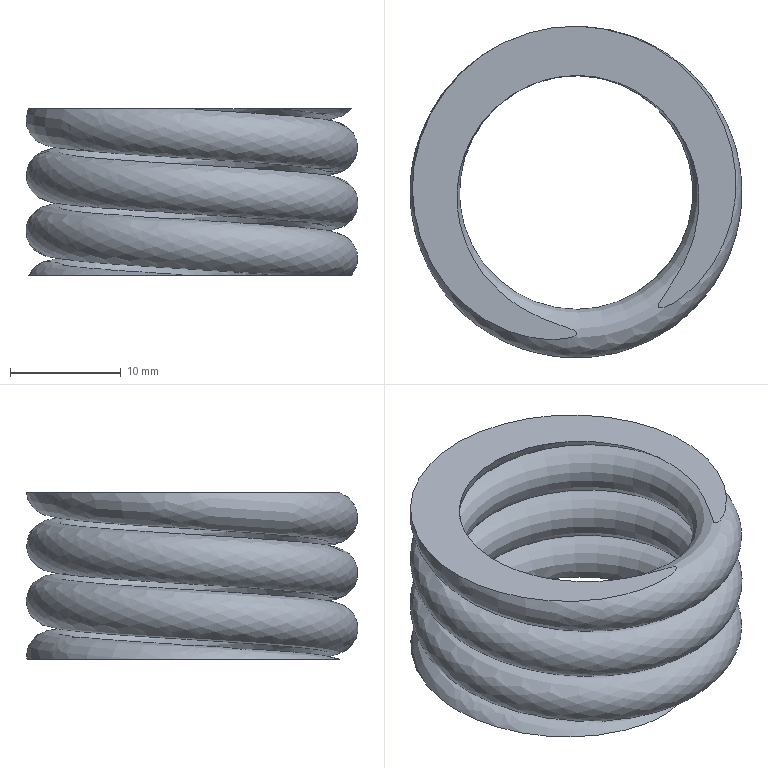Part | NX | features solid 2 | 1 solid | 3 faces | volume 3635 mm3 | plane 2 | spline 1
STEP:
#1=CARTESIAN_POINT('',(726.264,-215.262,-70.));
#2=VERTEX_POINT('',#1);
#3=CARTESIAN_POINT('',(727.992,-218.675,-70.));
#4=CARTESIAN_POINT('',(726.532,-215.094,-70.));
#5=CARTESIAN_POINT('',(723.172,-211.808,-70.));
#6=CARTESIAN_POINT('',(717.311,-209.605,-70.));
#7=CARTESIAN_POINT('',(710.898,-211.435,-70.));
#8=CARTESIAN_POINT('',(707.097,-216.445,-70.));
#9=CARTESIAN_POINT('',(705.99,-220.997,-70.));
#10=CARTESIAN_POINT('',(706.678,-224.835,-70.));
#11=CARTESIAN_POINT('',(708.087,-227.589,-70.));
#12=CARTESIAN_POINT('',(709.526,-229.372,-70.));
#13=CARTESIAN_POINT('',(711.287,-230.877,-70.));
#14=CARTESIAN_POINT('',(712.937,-231.853,-70.));
#15=CARTESIAN_POINT('',(714.343,-232.482,-70.));
#16=CARTESIAN_POINT('',(715.247,-232.816,-70.));
#17=CARTESIAN_POINT('',(715.973,-233.068,-70.));
#18=CARTESIAN_POINT('',(716.432,-233.226,-70.));
#19=CARTESIAN_POINT('',(716.774,-233.384,-70.));
#20=CARTESIAN_POINT('',(717.061,-233.517,-70.));
#21=CARTESIAN_POINT('',(717.084,-233.836,-70.));
#22=CARTESIAN_POINT('',(716.69,-234.013,-70.));
#23=CARTESIAN_POINT('',(716.256,-234.14,-70.));
#24=CARTESIAN_POINT('',(715.493,-234.247,-70.));
#25=CARTESIAN_POINT('',(714.56,-234.264,-70.));
#26=CARTESIAN_POINT('',(713.423,-234.146,-70.));
#27=CARTESIAN_POINT('',(711.959,-233.836,-70.));
#28=CARTESIAN_POINT('',(710.183,-233.184,-70.));
#29=CARTESIAN_POINT('',(708.231,-232.057,-70.));
#30=CARTESIAN_POINT('',(706.474,-230.61,-70.));
#31=CARTESIAN_POINT('',(704.512,-228.354,-70.));
#32=CARTESIAN_POINT('',(702.813,-224.942,-70.));
#33=CARTESIAN_POINT('',(702.119,-220.444,-70.));
#34=CARTESIAN_POINT('',(702.878,-215.95,-70.));
#35=CARTESIAN_POINT('',(704.967,-211.904,-70.));
#36=CARTESIAN_POINT('',(709.229,-207.583,-70.));
#37=CARTESIAN_POINT('',(715.189,-205.56,-70.));
#38=CARTESIAN_POINT('',(721.186,-206.381,-70.));
#39=CARTESIAN_POINT('',(725.307,-208.325,-70.));
#40=CARTESIAN_POINT('',(728.636,-211.403,-70.));
#41=CARTESIAN_POINT('',(730.838,-215.399,-70.));
#42=CARTESIAN_POINT('',(731.587,-219.101,-70.));
#43=CARTESIAN_POINT('',(731.42,-222.132,-70.));
#44=CARTESIAN_POINT('',(730.929,-224.311,-70.));
#45=CARTESIAN_POINT('',(730.067,-226.425,-70.));
#46=CARTESIAN_POINT('',(729.079,-228.001,-70.));
#47=CARTESIAN_POINT('',(728.109,-229.155,-70.));
#48=CARTESIAN_POINT('',(727.29,-229.946,-70.));
#49=CARTESIAN_POINT('',(726.539,-230.522,-70.));
#50=CARTESIAN_POINT('',(725.89,-230.918,-70.));
#51=CARTESIAN_POINT('',(725.467,-231.13,-70.));
#52=CARTESIAN_POINT('',(725.105,-231.262,-70.));
#53=CARTESIAN_POINT('',(724.844,-231.332,-70.));
#54=CARTESIAN_POINT('',(724.491,-231.323,-70.));
#55=CARTESIAN_POINT('',(724.529,-230.977,-70.));
#56=CARTESIAN_POINT('',(724.67,-230.741,-70.));
#57=CARTESIAN_POINT('',(724.871,-230.417,-70.));
#58=CARTESIAN_POINT('',(725.147,-230.034,-70.));
#59=CARTESIAN_POINT('',(725.476,-229.571,-70.));
#60=CARTESIAN_POINT('',(725.906,-228.948,-70.));
#61=CARTESIAN_POINT('',(726.408,-228.149,-70.));
#62=CARTESIAN_POINT('',(726.936,-227.149,-70.));
#63=CARTESIAN_POINT('',(727.536,-225.747,-70.));
#64=CARTESIAN_POINT('',(728.052,-223.943,-70.));
#65=CARTESIAN_POINT('',(728.282,-221.66,-70.));
#66=CARTESIAN_POINT('',(727.992,-218.675,-70.));
#67=CARTESIAN_POINT('',(726.532,-215.094,-70.));
#68=CARTESIAN_POINT('',(723.172,-211.808,-70.));
#69=B_SPLINE_CURVE_WITH_KNOTS('',3,(#3,#4,#5,#6,#7,#8,#9,#10,#11,#12,#13,#14,#15,#16,#17,#18,#19,#20,#21,#22,#23,#24,#25,#26,#27,#28,#29,#30,#31,#32,#33,#34,#35,#36,#37,#38,#39,#40,#41,#42,#43,#44,#45,#46,#47,#48,#49,#50,#51,#52,#53,#54,#55,#56,#57,#58,#59,#60,#61,#62,#63,#64,#65,#66,#67,#68),.UNSPECIFIED.,.T.,.F.,(1,1,1,1,1,1,1,1,1,1,1,1,1,1,1,1,1,1,1,1,1,1,1,1,1,1,1,1,1,1,1,1,1,1,1,1,1,1,1,1,1,1,1,1,1,1,1,1,1,1,1,1,1,1,1,1,1,1,1,1,1,1,1,1,1,1,1,1,1,1),(-0.009133,-0.00685,-0.004566,0.,0.004566,0.009133,0.01827,0.02283,0.0274,0.03197,0.03425,0.03653,0.03882,0.0411,0.04224,0.04338,0.04395,0.04452,0.04481,0.04509,0.04538,0.04566,0.04624,0.04681,0.04795,0.04909,0.05023,0.05251,0.0548,0.05708,0.05936,0.06393,0.0685,0.07306,0.07763,0.0822,0.09133,0.0959,0.1005,0.105,0.1096,0.1142,0.1164,0.1187,0.121,0.1233,0.1244,0.1256,0.1267,0.1273,0.1279,0.1281,0.1284,0.1287,0.129,0.1293,0.1296,0.1301,0.1307,0.1313,0.1324,0.1336,0.1347,0.137,0.1393,0.1416,0.1461,0.1507,0.1553,0.1644),.UNSPECIFIED.);
#70=EDGE_CURVE('',#2,#2,#69,.T.);
#71=ORIENTED_EDGE('',*,*,#70,.T.);
#72=EDGE_LOOP('',(#71));
#73=FACE_BOUND('',#72,.T.);
#74=CARTESIAN_POINT('',(717.081,-220.938,-70.));
#75=DIRECTION('',(0.,0.,-1.));
#76=DIRECTION('',(1.,0.,0.));
#77=AXIS2_PLACEMENT_3D('',#74,#75,#76);
#78=PLANE('',#77);
#79=ADVANCED_FACE('',(#73),#78,.T.);
#80=CARTESIAN_POINT('',(724.49,-231.227,-55.));
#81=VERTEX_POINT('',#80);
#82=CARTESIAN_POINT('',(724.724,-231.392,-55.));
#83=CARTESIAN_POINT('',(724.417,-231.259,-55.));
#84=CARTESIAN_POINT('',(724.55,-230.935,-55.));
#85=CARTESIAN_POINT('',(724.729,-230.617,-55.));
#86=CARTESIAN_POINT('',(725.006,-230.215,-55.));
#87=CARTESIAN_POINT('',(725.336,-229.748,-55.));
#88=CARTESIAN_POINT('',(725.772,-229.118,-55.));
#89=CARTESIAN_POINT('',(726.285,-228.313,-55.));
#90=CARTESIAN_POINT('',(727.013,-226.979,-55.));
#91=CARTESIAN_POINT('',(727.733,-225.182,-55.));
#92=CARTESIAN_POINT('',(728.186,-222.958,-55.));
#93=CARTESIAN_POINT('',(728.213,-220.644,-55.));
#94=CARTESIAN_POINT('',(727.644,-217.647,-55.));
#95=CARTESIAN_POINT('',(725.827,-214.184,-55.));
#96=CARTESIAN_POINT('',(722.16,-211.277,-55.));
#97=CARTESIAN_POINT('',(717.607,-210.079,-55.));
#98=CARTESIAN_POINT('',(713.,-210.916,-55.));
#99=CARTESIAN_POINT('',(709.112,-213.524,-55.));
#100=CARTESIAN_POINT('',(706.667,-217.549,-55.));
#101=CARTESIAN_POINT('',(706.042,-222.19,-55.));
#102=CARTESIAN_POINT('',(707.124,-225.938,-55.));
#103=CARTESIAN_POINT('',(708.796,-228.526,-55.));
#104=CARTESIAN_POINT('',(710.39,-230.176,-55.));
#105=CARTESIAN_POINT('',(711.965,-231.296,-55.));
#106=CARTESIAN_POINT('',(713.318,-232.015,-55.));
#107=CARTESIAN_POINT('',(714.374,-232.478,-55.));
#108=CARTESIAN_POINT('',(715.28,-232.807,-55.));
#109=CARTESIAN_POINT('',(716.008,-233.055,-55.));
#110=CARTESIAN_POINT('',(716.467,-233.208,-55.));
#111=CARTESIAN_POINT('',(716.814,-233.362,-55.));
#112=CARTESIAN_POINT('',(717.096,-233.482,-55.));
#113=CARTESIAN_POINT('',(717.179,-233.795,-55.));
#114=CARTESIAN_POINT('',(716.777,-233.987,-55.));
#115=CARTESIAN_POINT('',(716.348,-234.111,-55.));
#116=CARTESIAN_POINT('',(715.773,-234.195,-55.));
#117=CARTESIAN_POINT('',(715.209,-234.23,-55.));
#118=CARTESIAN_POINT('',(714.457,-234.228,-55.));
#119=CARTESIAN_POINT('',(713.145,-234.109,-55.));
#120=CARTESIAN_POINT('',(711.303,-233.659,-55.));
#121=CARTESIAN_POINT('',(709.245,-232.739,-55.));
#122=CARTESIAN_POINT('',(707.369,-231.464,-55.));
#123=CARTESIAN_POINT('',(705.74,-229.891,-55.));
#124=CARTESIAN_POINT('',(703.959,-227.463,-55.));
#125=CARTESIAN_POINT('',(702.501,-223.95,-55.));
#126=CARTESIAN_POINT('',(702.127,-219.407,-55.));
#127=CARTESIAN_POINT('',(703.573,-213.5,-55.));
#128=CARTESIAN_POINT('',(708.594,-207.481,-55.));
#129=CARTESIAN_POINT('',(716.197,-205.431,-55.));
#130=CARTESIAN_POINT('',(722.139,-206.68,-55.));
#131=CARTESIAN_POINT('',(726.131,-208.866,-55.));
#132=CARTESIAN_POINT('',(729.237,-212.198,-55.));
#133=CARTESIAN_POINT('',(731.181,-216.325,-55.));
#134=CARTESIAN_POINT('',(731.661,-220.084,-55.));
#135=CARTESIAN_POINT('',(731.274,-223.089,-55.));
#136=CARTESIAN_POINT('',(730.618,-225.234,-55.));
#137=CARTESIAN_POINT('',(729.589,-227.263,-55.));
#138=CARTESIAN_POINT('',(728.465,-228.762,-55.));
#139=CARTESIAN_POINT('',(727.41,-229.822,-55.));
#140=CARTESIAN_POINT('',(726.671,-230.423,-55.));
#141=CARTESIAN_POINT('',(726.036,-230.841,-55.));
#142=CARTESIAN_POINT('',(725.536,-231.119,-55.));
#143=CARTESIAN_POINT('',(725.092,-231.289,-55.));
#144=CARTESIAN_POINT('',(724.724,-231.392,-55.));
#145=CARTESIAN_POINT('',(724.417,-231.259,-55.));
#146=CARTESIAN_POINT('',(724.55,-230.935,-55.));
#147=B_SPLINE_CURVE_WITH_KNOTS('',3,(#82,#83,#84,#85,#86,#87,#88,#89,#90,#91,#92,#93,#94,#95,#96,#97,#98,#99,#100,#101,#102,#103,#104,#105,#106,#107,#108,#109,#110,#111,#112,#113,#114,#115,#116,#117,#118,#119,#120,#121,#122,#123,#124,#125,#126,#127,#128,#129,#130,#131,#132,#133,#134,#135,#136,#137,#138,#139,#140,#141,#142,#143,#144,#145,#146),.UNSPECIFIED.,.T.,.F.,(1,1,1,1,1,1,1,1,1,1,1,1,1,1,1,1,1,1,1,1,1,1,1,1,1,1,1,1,1,1,1,1,1,1,1,1,1,1,1,1,1,1,1,1,1,1,1,1,1,1,1,1,1,1,1,1,1,1,1,1,1,1,1,1,1,1,1,1,1),(-0.001153,-0.0005764,-0.0002882,0.,0.0002882,0.0005764,0.001153,0.001729,0.002306,0.003458,0.004611,0.006917,0.009222,0.01153,0.01383,0.01844,0.02306,0.02767,0.03228,0.03689,0.0415,0.04611,0.05072,0.05303,0.05533,0.05764,0.05879,0.05995,0.0611,0.06168,0.06225,0.06254,0.06283,0.06312,0.0634,0.06398,0.06456,0.06513,0.06571,0.06686,0.06917,0.07147,0.07378,0.07609,0.07839,0.083,0.08761,0.09222,0.1014,0.1107,0.1153,0.1199,0.1245,0.1291,0.1337,0.136,0.1383,0.1406,0.1429,0.1441,0.1453,0.1458,0.1464,0.147,0.1473,0.1476,0.1478,0.1481,0.1487),.UNSPECIFIED.);
#148=EDGE_CURVE('',#81,#81,#147,.T.);
#149=ORIENTED_EDGE('',*,*,#148,.T.);
#150=EDGE_LOOP('',(#149));
#151=FACE_BOUND('',#150,.T.);
#152=ORIENTED_EDGE('',*,*,#70,.F.);
#153=EDGE_LOOP('',(#152));
#154=FACE_BOUND('',#153,.T.);
#155=CARTESIAN_POINT('',(718.446,-231.593,-73.635));
#156=CARTESIAN_POINT('',(718.399,-231.599,-73.632));
#157=CARTESIAN_POINT('',(717.039,-231.776,-73.546));
#158=CARTESIAN_POINT('',(712.928,-231.512,-73.292));
#159=CARTESIAN_POINT('',(707.15,-227.471,-72.88));
#160=CARTESIAN_POINT('',(705.263,-219.102,-72.379));
#161=CARTESIAN_POINT('',(709.524,-211.573,-71.875));
#162=CARTESIAN_POINT('',(717.773,-208.836,-71.368));
#163=CARTESIAN_POINT('',(725.78,-212.39,-70.857));
#164=CARTESIAN_POINT('',(729.36,-220.451,-70.343));
#165=CARTESIAN_POINT('',(726.568,-228.872,-69.825));
#166=CARTESIAN_POINT('',(718.78,-233.281,-69.303));
#167=CARTESIAN_POINT('',(710.001,-231.303,-68.777));
#168=CARTESIAN_POINT('',(705.698,-225.153,-68.339));
#169=CARTESIAN_POINT('',(705.325,-219.36,-67.982));
#170=CARTESIAN_POINT('',(706.661,-215.22,-67.715));
#171=CARTESIAN_POINT('',(709.368,-211.795,-67.447));
#172=CARTESIAN_POINT('',(713.171,-209.612,-67.178));
#173=CARTESIAN_POINT('',(717.512,-208.877,-66.907));
#174=CARTESIAN_POINT('',(721.829,-209.829,-66.636));
#175=CARTESIAN_POINT('',(725.57,-212.222,-66.363));
#176=CARTESIAN_POINT('',(728.154,-215.854,-66.089));
#177=CARTESIAN_POINT('',(729.329,-220.176,-65.814));
#178=CARTESIAN_POINT('',(728.805,-224.64,-65.538));
#179=CARTESIAN_POINT('',(726.743,-228.659,-65.261));
#180=CARTESIAN_POINT('',(722.187,-232.668,-64.888));
#181=CARTESIAN_POINT('',(714.328,-234.064,-64.421));
#182=CARTESIAN_POINT('',(706.146,-228.881,-63.856));
#183=CARTESIAN_POINT('',(703.52,-219.454,-63.285));
#184=CARTESIAN_POINT('',(707.951,-210.653,-62.71));
#185=CARTESIAN_POINT('',(717.228,-207.065,-62.13));
#186=CARTESIAN_POINT('',(726.583,-210.682,-61.545));
#187=CARTESIAN_POINT('',(731.127,-219.703,-60.956));
#188=CARTESIAN_POINT('',(728.392,-229.525,-60.361));
#189=CARTESIAN_POINT('',(719.724,-235.018,-59.762));
#190=CARTESIAN_POINT('',(711.249,-233.514,-59.259));
#191=CARTESIAN_POINT('',(706.304,-229.164,-58.854));
#192=CARTESIAN_POINT('',(704.036,-224.745,-58.55));
#193=CARTESIAN_POINT('',(703.453,-219.789,-58.242));
#194=CARTESIAN_POINT('',(704.766,-214.957,-57.935));
#195=CARTESIAN_POINT('',(707.68,-210.86,-57.626));
#196=CARTESIAN_POINT('',(711.931,-208.141,-57.317));
#197=CARTESIAN_POINT('',(716.879,-207.048,-57.006));
#198=CARTESIAN_POINT('',(721.893,-207.897,-56.693));
#199=CARTESIAN_POINT('',(726.319,-210.437,-56.38));
#200=CARTESIAN_POINT('',(729.495,-214.455,-56.065));
#201=CARTESIAN_POINT('',(731.075,-219.345,-55.75));
#202=CARTESIAN_POINT('',(730.636,-226.188,-55.328));
#203=CARTESIAN_POINT('',(727.222,-231.068,-54.98));
#204=CARTESIAN_POINT('',(723.893,-233.05,-54.738));
#205=CARTESIAN_POINT('',(723.48,-233.269,-54.708));
#206=CARTESIAN_POINT('',(718.494,-231.227,-72.09));
#207=CARTESIAN_POINT('',(718.449,-231.234,-72.087));
#208=CARTESIAN_POINT('',(717.132,-231.406,-72.005));
#209=CARTESIAN_POINT('',(713.156,-231.15,-71.759));
#210=CARTESIAN_POINT('',(707.615,-227.274,-71.364));
#211=CARTESIAN_POINT('',(705.811,-219.277,-70.885));
#212=CARTESIAN_POINT('',(709.859,-212.125,-70.406));
#213=CARTESIAN_POINT('',(717.649,-209.54,-69.927));
#214=CARTESIAN_POINT('',(725.168,-212.878,-69.448));
#215=CARTESIAN_POINT('',(728.511,-220.407,-68.967));
#216=CARTESIAN_POINT('',(725.918,-228.229,-68.486));
#217=CARTESIAN_POINT('',(718.718,-232.305,-68.004));
#218=CARTESIAN_POINT('',(710.644,-230.486,-67.521));
#219=CARTESIAN_POINT('',(706.719,-224.876,-67.12));
#220=CARTESIAN_POINT('',(706.376,-219.566,-66.793));
#221=CARTESIAN_POINT('',(707.592,-215.8,-66.551));
#222=CARTESIAN_POINT('',(710.048,-212.693,-66.307));
#223=CARTESIAN_POINT('',(713.493,-210.715,-66.063));
#224=CARTESIAN_POINT('',(717.415,-210.051,-65.819));
#225=CARTESIAN_POINT('',(721.309,-210.91,-65.574));
#226=CARTESIAN_POINT('',(724.678,-213.065,-65.329));
#227=CARTESIAN_POINT('',(727.001,-216.33,-65.082));
#228=CARTESIAN_POINT('',(728.056,-220.209,-64.836));
#229=CARTESIAN_POINT('',(727.586,-224.207,-64.588));
#230=CARTESIAN_POINT('',(725.74,-227.806,-64.34));
#231=CARTESIAN_POINT('',(721.643,-231.411,-64.005));
#232=CARTESIAN_POINT('',(714.659,-232.652,-63.59));
#233=CARTESIAN_POINT('',(707.368,-228.033,-63.086));
#234=CARTESIAN_POINT('',(705.032,-219.646,-62.578));
#235=CARTESIAN_POINT('',(708.966,-211.832,-62.068));
#236=CARTESIAN_POINT('',(717.192,-208.65,-61.553));
#237=CARTESIAN_POINT('',(725.478,-211.853,-61.036));
#238=CARTESIAN_POINT('',(729.497,-219.834,-60.514));
#239=CARTESIAN_POINT('',(727.079,-228.521,-59.988));
#240=CARTESIAN_POINT('',(719.42,-233.374,-59.459));
#241=CARTESIAN_POINT('',(711.969,-232.052,-59.016));
#242=CARTESIAN_POINT('',(707.577,-228.189,-58.657));
#243=CARTESIAN_POINT('',(705.574,-224.287,-58.388));
#244=CARTESIAN_POINT('',(705.06,-219.916,-58.117));
#245=CARTESIAN_POINT('',(706.219,-215.65,-57.846));
#246=CARTESIAN_POINT('',(708.792,-212.033,-57.573));
#247=CARTESIAN_POINT('',(712.548,-209.631,-57.3));
#248=CARTESIAN_POINT('',(716.92,-208.665,-57.025));
#249=CARTESIAN_POINT('',(721.352,-209.416,-56.748));
#250=CARTESIAN_POINT('',(725.269,-211.663,-56.471));
#251=CARTESIAN_POINT('',(728.081,-215.22,-56.193));
#252=CARTESIAN_POINT('',(729.481,-219.554,-55.913));
#253=CARTESIAN_POINT('',(729.089,-225.659,-55.537));
#254=CARTESIAN_POINT('',(726.067,-229.98,-55.229));
#255=CARTESIAN_POINT('',(723.108,-231.737,-55.014));
#256=CARTESIAN_POINT('',(722.74,-231.931,-54.988));
#257=CARTESIAN_POINT('',(718.586,-231.366,-70.976));
#258=CARTESIAN_POINT('',(718.54,-231.372,-70.973));
#259=CARTESIAN_POINT('',(717.205,-231.547,-70.889));
#260=CARTESIAN_POINT('',(713.181,-231.289,-70.64));
#261=CARTESIAN_POINT('',(707.588,-227.377,-70.242));
#262=CARTESIAN_POINT('',(705.776,-219.343,-69.76));
#263=CARTESIAN_POINT('',(709.823,-212.192,-69.282));
#264=CARTESIAN_POINT('',(717.574,-209.621,-68.805));
#265=CARTESIAN_POINT('',(725.021,-212.926,-68.33));
#266=CARTESIAN_POINT('',(728.316,-220.347,-67.857));
#267=CARTESIAN_POINT('',(725.772,-228.02,-67.385));
#268=CARTESIAN_POINT('',(718.741,-232.001,-66.914));
#269=CARTESIAN_POINT('',(710.895,-230.232,-66.444));
#270=CARTESIAN_POINT('',(707.102,-224.811,-66.057));
#271=CARTESIAN_POINT('',(706.772,-219.681,-65.741));
#272=CARTESIAN_POINT('',(707.941,-216.06,-65.508));
#273=CARTESIAN_POINT('',(710.296,-213.08,-65.274));
#274=CARTESIAN_POINT('',(713.595,-211.187,-65.041));
#275=CARTESIAN_POINT('',(717.339,-210.552,-64.807));
#276=CARTESIAN_POINT('',(721.05,-211.371,-64.574));
#277=CARTESIAN_POINT('',(724.255,-213.42,-64.341));
#278=CARTESIAN_POINT('',(726.46,-216.519,-64.107));
#279=CARTESIAN_POINT('',(727.458,-220.193,-63.873));
#280=CARTESIAN_POINT('',(727.015,-223.972,-63.639));
#281=CARTESIAN_POINT('',(725.273,-227.367,-63.406));
#282=CARTESIAN_POINT('',(721.4,-230.775,-63.088));
#283=CARTESIAN_POINT('',(714.857,-231.937,-62.7));
#284=CARTESIAN_POINT('',(708.026,-227.61,-62.227));
#285=CARTESIAN_POINT('',(705.844,-219.778,-61.754));
#286=CARTESIAN_POINT('',(709.507,-212.502,-61.278));
#287=CARTESIAN_POINT('',(717.145,-209.548,-60.801));
#288=CARTESIAN_POINT('',(724.818,-212.514,-60.321));
#289=CARTESIAN_POINT('',(728.531,-219.887,-59.839));
#290=CARTESIAN_POINT('',(726.302,-227.894,-59.355));
#291=CARTESIAN_POINT('',(719.257,-232.358,-58.868));
#292=CARTESIAN_POINT('',(712.442,-231.149,-58.463));
#293=CARTESIAN_POINT('',(708.397,-227.591,-58.132));
#294=CARTESIAN_POINT('',(706.564,-224.019,-57.886));
#295=CARTESIAN_POINT('',(706.094,-220.023,-57.638));
#296=CARTESIAN_POINT('',(707.154,-216.124,-57.39));
#297=CARTESIAN_POINT('',(709.504,-212.819,-57.141));
#298=CARTESIAN_POINT('',(712.933,-210.626,-56.891));
#299=CARTESIAN_POINT('',(716.923,-209.745,-56.64));
#300=CARTESIAN_POINT('',(720.965,-210.429,-56.388));
#301=CARTESIAN_POINT('',(724.538,-212.48,-56.136));
#302=CARTESIAN_POINT('',(727.101,-215.721,-55.882));
#303=CARTESIAN_POINT('',(728.378,-219.674,-55.627));
#304=CARTESIAN_POINT('',(728.018,-225.267,-55.282));
#305=CARTESIAN_POINT('',(725.272,-229.194,-55.002));
#306=CARTESIAN_POINT('',(722.575,-230.793,-54.806));
#307=CARTESIAN_POINT('',(722.24,-230.969,-54.782));
#308=CARTESIAN_POINT('',(718.755,-232.288,-70.353));
#309=CARTESIAN_POINT('',(718.706,-232.295,-70.35));
#310=CARTESIAN_POINT('',(717.257,-232.485,-70.258));
#311=CARTESIAN_POINT('',(712.903,-232.205,-69.99));
#312=CARTESIAN_POINT('',(706.815,-227.947,-69.556));
#313=CARTESIAN_POINT('',(704.854,-219.253,-69.035));
#314=CARTESIAN_POINT('',(709.222,-211.536,-68.518));
#315=CARTESIAN_POINT('',(717.566,-208.767,-68.005));
#316=CARTESIAN_POINT('',(725.559,-212.315,-67.495));
#317=CARTESIAN_POINT('',(729.084,-220.255,-66.989));
#318=CARTESIAN_POINT('',(726.371,-228.439,-66.485));
#319=CARTESIAN_POINT('',(718.899,-232.669,-65.985));
#320=CARTESIAN_POINT('',(710.589,-230.797,-65.487));
#321=CARTESIAN_POINT('',(706.575,-225.061,-65.078));
#322=CARTESIAN_POINT('',(706.229,-219.676,-64.746));
#323=CARTESIAN_POINT('',(707.457,-215.872,-64.501));
#324=CARTESIAN_POINT('',(709.926,-212.748,-64.256));
#325=CARTESIAN_POINT('',(713.376,-210.768,-64.012));
#326=CARTESIAN_POINT('',(717.285,-210.105,-63.769));
#327=CARTESIAN_POINT('',(721.151,-210.958,-63.526));
#328=CARTESIAN_POINT('',(724.48,-213.087,-63.283));
#329=CARTESIAN_POINT('',(726.766,-216.3,-63.041));
#330=CARTESIAN_POINT('',(727.799,-220.1,-62.799));
#331=CARTESIAN_POINT('',(727.341,-224.,-62.558));
#332=CARTESIAN_POINT('',(725.548,-227.496,-62.317));
#333=CARTESIAN_POINT('',(721.578,-230.989,-61.992));
#334=CARTESIAN_POINT('',(714.88,-232.178,-61.594));
#335=CARTESIAN_POINT('',(707.925,-227.772,-61.113));
#336=CARTESIAN_POINT('',(705.714,-219.835,-60.633));
#337=CARTESIAN_POINT('',(709.408,-212.498,-60.153));
#338=CARTESIAN_POINT('',(717.075,-209.532,-59.674));
#339=CARTESIAN_POINT('',(724.74,-212.496,-59.195));
#340=CARTESIAN_POINT('',(728.432,-219.826,-58.716));
#341=CARTESIAN_POINT('',(726.225,-227.75,-58.236));
#342=CARTESIAN_POINT('',(719.286,-232.147,-57.757));
#343=CARTESIAN_POINT('',(712.608,-230.962,-57.36));
#344=CARTESIAN_POINT('',(708.65,-227.481,-57.036));
#345=CARTESIAN_POINT('',(706.863,-223.999,-56.796));
#346=CARTESIAN_POINT('',(706.406,-220.114,-56.555));
#347=CARTESIAN_POINT('',(707.434,-216.331,-56.315));
#348=CARTESIAN_POINT('',(709.709,-213.132,-56.074));
#349=CARTESIAN_POINT('',(713.022,-211.013,-55.832));
#350=CARTESIAN_POINT('',(716.867,-210.164,-55.591));
#351=CARTESIAN_POINT('',(720.755,-210.822,-55.348));
#352=CARTESIAN_POINT('',(724.185,-212.79,-55.106));
#353=CARTESIAN_POINT('',(726.64,-215.895,-54.862));
#354=CARTESIAN_POINT('',(727.861,-219.675,-54.619));
#355=CARTESIAN_POINT('',(727.517,-225.026,-54.289));
#356=CARTESIAN_POINT('',(724.908,-228.756,-54.023));
#357=CARTESIAN_POINT('',(722.349,-230.274,-53.837));
#358=CARTESIAN_POINT('',(722.031,-230.441,-53.814));
#359=CARTESIAN_POINT('',(718.993,-233.813,-69.996));
#360=CARTESIAN_POINT('',(718.937,-233.821,-69.993));
#361=CARTESIAN_POINT('',(717.301,-234.037,-69.89));
#362=CARTESIAN_POINT('',(712.398,-233.722,-69.587));
#363=CARTESIAN_POINT('',(705.476,-228.881,-69.094));
#364=CARTESIAN_POINT('',(703.259,-219.051,-68.505));
#365=CARTESIAN_POINT('',(708.19,-210.339,-67.922));
#366=CARTESIAN_POINT('',(717.6,-207.217,-67.343));
#367=CARTESIAN_POINT('',(726.598,-211.211,-66.769));
#368=CARTESIAN_POINT('',(730.56,-220.133,-66.2));
#369=CARTESIAN_POINT('',(727.517,-229.312,-65.635));
#370=CARTESIAN_POINT('',(719.16,-234.044,-65.076));
#371=CARTESIAN_POINT('',(709.886,-231.954,-64.52));
#372=CARTESIAN_POINT('',(705.398,-225.541,-64.063));
#373=CARTESIAN_POINT('',(705.015,-219.591,-63.696));
#374=CARTESIAN_POINT('',(706.377,-215.372,-63.424));
#375=CARTESIAN_POINT('',(709.113,-211.911,-63.153));
#376=CARTESIAN_POINT('',(712.926,-209.722,-62.883));
#377=CARTESIAN_POINT('',(717.24,-208.991,-62.614));
#378=CARTESIAN_POINT('',(721.497,-209.93,-62.347));
#379=CARTESIAN_POINT('',(725.155,-212.269,-62.08));
#380=CARTESIAN_POINT('',(727.661,-215.792,-61.814));
#381=CARTESIAN_POINT('',(728.791,-219.948,-61.55));
#382=CARTESIAN_POINT('',(728.291,-224.207,-61.286));
#383=CARTESIAN_POINT('',(726.34,-228.01,-61.025));
#384=CARTESIAN_POINT('',(722.052,-231.783,-60.673));
#385=CARTESIAN_POINT('',(714.79,-233.073,-60.242));
#386=CARTESIAN_POINT('',(707.312,-228.336,-59.725));
#387=CARTESIAN_POINT('',(704.948,-219.85,-59.212));
#388=CARTESIAN_POINT('',(708.877,-212.047,-58.702));
#389=CARTESIAN_POINT('',(716.983,-208.912,-58.195));
#390=CARTESIAN_POINT('',(725.039,-212.026,-57.692));
#391=CARTESIAN_POINT('',(728.896,-219.684,-57.191));
#392=CARTESIAN_POINT('',(726.605,-227.912,-56.693));
#393=CARTESIAN_POINT('',(719.445,-232.449,-56.198));
#394=CARTESIAN_POINT('',(712.587,-231.232,-55.791));
#395=CARTESIAN_POINT('',(708.551,-227.682,-55.46));
#396=CARTESIAN_POINT('',(706.734,-224.141,-55.217));
#397=CARTESIAN_POINT('',(706.271,-220.204,-54.973));
#398=CARTESIAN_POINT('',(707.31,-216.381,-54.73));
#399=CARTESIAN_POINT('',(709.6,-213.161,-54.487));
#400=CARTESIAN_POINT('',(712.924,-211.035,-54.245));
#401=CARTESIAN_POINT('',(716.768,-210.186,-54.003));
#402=CARTESIAN_POINT('',(720.643,-210.842,-53.761));
#403=CARTESIAN_POINT('',(724.049,-212.796,-53.521));
#404=CARTESIAN_POINT('',(726.479,-215.87,-53.28));
#405=CARTESIAN_POINT('',(727.683,-219.598,-53.039));
#406=CARTESIAN_POINT('',(727.345,-224.862,-52.715));
#407=CARTESIAN_POINT('',(724.796,-228.505,-52.455));
#408=CARTESIAN_POINT('',(722.304,-229.987,-52.274));
#409=CARTESIAN_POINT('',(721.995,-230.15,-52.252));
#410=CARTESIAN_POINT('',(719.139,-234.917,-70.145));
#411=CARTESIAN_POINT('',(719.078,-234.926,-70.142));
#412=CARTESIAN_POINT('',(717.306,-235.16,-70.03));
#413=CARTESIAN_POINT('',(712.005,-234.82,-69.703));
#414=CARTESIAN_POINT('',(704.471,-229.55,-69.166));
#415=CARTESIAN_POINT('',(702.063,-218.873,-68.526));
#416=CARTESIAN_POINT('',(707.42,-209.406,-67.892));
#417=CARTESIAN_POINT('',(717.654,-206.011,-67.263));
#418=CARTESIAN_POINT('',(727.442,-210.356,-66.639));
#419=CARTESIAN_POINT('',(731.753,-220.064,-66.02));
#420=CARTESIAN_POINT('',(728.44,-230.053,-65.405));
#421=CARTESIAN_POINT('',(719.348,-235.201,-64.796));
#422=CARTESIAN_POINT('',(709.258,-232.926,-64.192));
#423=CARTESIAN_POINT('',(704.361,-225.929,-63.693));
#424=CARTESIAN_POINT('',(703.946,-219.483,-63.295));
#425=CARTESIAN_POINT('',(705.428,-214.895,-63.));
#426=CARTESIAN_POINT('',(708.403,-211.13,-62.705));
#427=CARTESIAN_POINT('',(712.547,-208.752,-62.412));
#428=CARTESIAN_POINT('',(717.235,-207.957,-62.12));
#429=CARTESIAN_POINT('',(721.858,-208.977,-61.829));
#430=CARTESIAN_POINT('',(725.826,-211.515,-61.54));
#431=CARTESIAN_POINT('',(728.544,-215.336,-61.252));
#432=CARTESIAN_POINT('',(729.769,-219.839,-60.965));
#433=CARTESIAN_POINT('',(729.227,-224.452,-60.68));
#434=CARTESIAN_POINT('',(727.117,-228.565,-60.396));
#435=CARTESIAN_POINT('',(722.503,-232.625,-60.019));
#436=CARTESIAN_POINT('',(714.648,-234.02,-59.552));
#437=CARTESIAN_POINT('',(706.6,-228.922,-58.996));
#438=CARTESIAN_POINT('',(704.062,-219.811,-58.444));
#439=CARTESIAN_POINT('',(708.27,-211.453,-57.898));
#440=CARTESIAN_POINT('',(716.93,-208.103,-57.357));
#441=CARTESIAN_POINT('',(725.513,-211.422,-56.82));
#442=CARTESIAN_POINT('',(729.611,-219.558,-56.289));
#443=CARTESIAN_POINT('',(727.185,-228.271,-55.761));
#444=CARTESIAN_POINT('',(719.627,-233.06,-55.239));
#445=CARTESIAN_POINT('',(712.392,-231.776,-54.809));
#446=CARTESIAN_POINT('',(708.168,-228.06,-54.463));
#447=CARTESIAN_POINT('',(706.264,-224.35,-54.208));
#448=CARTESIAN_POINT('',(705.779,-220.231,-53.952));
#449=CARTESIAN_POINT('',(706.864,-216.241,-53.699));
#450=CARTESIAN_POINT('',(709.249,-212.887,-53.446));
#451=CARTESIAN_POINT('',(712.705,-210.677,-53.194));
#452=CARTESIAN_POINT('',(716.692,-209.796,-52.943));
#453=CARTESIAN_POINT('',(720.703,-210.475,-52.693));
#454=CARTESIAN_POINT('',(724.221,-212.494,-52.445));
#455=CARTESIAN_POINT('',(726.725,-215.661,-52.196));
#456=CARTESIAN_POINT('',(727.964,-219.494,-51.95));
#457=CARTESIAN_POINT('',(727.617,-224.885,-51.617));
#458=CARTESIAN_POINT('',(725.011,-228.611,-51.351));
#459=CARTESIAN_POINT('',(722.471,-230.124,-51.166));
#460=CARTESIAN_POINT('',(722.156,-230.291,-51.144));
#461=CARTESIAN_POINT('',(719.166,-235.541,-71.082));
#462=CARTESIAN_POINT('',(719.103,-235.55,-71.078));
#463=CARTESIAN_POINT('',(717.255,-235.794,-70.962));
#464=CARTESIAN_POINT('',(711.727,-235.439,-70.621));
#465=CARTESIAN_POINT('',(703.828,-229.914,-70.057));
#466=CARTESIAN_POINT('',(701.3,-218.706,-69.386));
#467=CARTESIAN_POINT('',(706.94,-208.74,-68.719));
#468=CARTESIAN_POINT('',(717.745,-205.156,-68.054));
#469=CARTESIAN_POINT('',(728.108,-209.755,-67.393));
#470=CARTESIAN_POINT('',(732.686,-220.063,-66.736));
#471=CARTESIAN_POINT('',(729.159,-230.698,-66.082));
#472=CARTESIAN_POINT('',(719.455,-236.192,-65.432));
#473=CARTESIAN_POINT('',(708.655,-233.758,-64.785));
#474=CARTESIAN_POINT('',(703.389,-226.233,-64.248));
#475=CARTESIAN_POINT('',(702.944,-219.325,-63.822));
#476=CARTESIAN_POINT('',(704.539,-214.385,-63.504));
#477=CARTESIAN_POINT('',(707.749,-210.325,-63.186));
#478=CARTESIAN_POINT('',(712.22,-207.758,-62.87));
#479=CARTESIAN_POINT('',(717.288,-206.899,-62.554));
#480=CARTESIAN_POINT('',(722.289,-208.003,-62.239));
#481=CARTESIAN_POINT('',(726.587,-210.75,-61.926));
#482=CARTESIAN_POINT('',(729.534,-214.892,-61.614));
#483=CARTESIAN_POINT('',(730.862,-219.779,-61.303));
#484=CARTESIAN_POINT('',(730.274,-224.791,-60.993));
#485=CARTESIAN_POINT('',(727.98,-229.261,-60.685));
#486=CARTESIAN_POINT('',(722.982,-233.658,-60.276));
#487=CARTESIAN_POINT('',(714.405,-235.182,-59.766));
#488=CARTESIAN_POINT('',(705.635,-229.626,-59.16));
#489=CARTESIAN_POINT('',(702.866,-219.687,-58.558));
#490=CARTESIAN_POINT('',(707.463,-210.557,-57.962));
#491=CARTESIAN_POINT('',(716.931,-206.895,-57.37));
#492=CARTESIAN_POINT('',(726.322,-210.526,-56.783));
#493=CARTESIAN_POINT('',(730.81,-219.435,-56.201));
#494=CARTESIAN_POINT('',(728.153,-228.978,-55.623));
#495=CARTESIAN_POINT('',(719.869,-234.227,-55.051));
#496=CARTESIAN_POINT('',(711.909,-232.814,-54.578));
#497=CARTESIAN_POINT('',(707.298,-228.759,-54.2));
#498=CARTESIAN_POINT('',(705.21,-224.69,-53.92));
#499=CARTESIAN_POINT('',(704.678,-220.169,-53.64));
#500=CARTESIAN_POINT('',(705.867,-215.793,-53.362));
#501=CARTESIAN_POINT('',(708.483,-212.115,-53.085));
#502=CARTESIAN_POINT('',(712.27,-209.693,-52.809));
#503=CARTESIAN_POINT('',(716.64,-208.728,-52.534));
#504=CARTESIAN_POINT('',(721.035,-209.472,-52.26));
#505=CARTESIAN_POINT('',(724.884,-211.681,-51.988));
#506=CARTESIAN_POINT('',(727.625,-215.147,-51.716));
#507=CARTESIAN_POINT('',(728.978,-219.336,-51.446));
#508=CARTESIAN_POINT('',(728.601,-225.195,-51.085));
#509=CARTESIAN_POINT('',(725.75,-229.271,-50.794));
#510=CARTESIAN_POINT('',(722.981,-230.925,-50.592));
#511=CARTESIAN_POINT('',(722.638,-231.106,-50.568));
#512=CARTESIAN_POINT('',(719.117,-235.906,-72.626));
#513=CARTESIAN_POINT('',(719.053,-235.915,-72.622));
#514=CARTESIAN_POINT('',(717.161,-236.165,-72.503));
#515=CARTESIAN_POINT('',(711.499,-235.802,-72.154));
#516=CARTESIAN_POINT('',(703.364,-230.111,-71.574));
#517=CARTESIAN_POINT('',(700.752,-218.53,-70.88));
#518=CARTESIAN_POINT('',(706.605,-208.188,-70.188));
#519=CARTESIAN_POINT('',(717.87,-204.451,-69.495));
#520=CARTESIAN_POINT('',(728.721,-209.267,-68.803));
#521=CARTESIAN_POINT('',(733.534,-220.108,-68.111));
#522=CARTESIAN_POINT('',(729.81,-231.341,-67.42));
#523=CARTESIAN_POINT('',(719.517,-237.168,-66.731));
#524=CARTESIAN_POINT('',(708.012,-234.576,-66.042));
#525=CARTESIAN_POINT('',(702.369,-226.511,-65.467));
#526=CARTESIAN_POINT('',(701.893,-219.119,-65.011));
#527=CARTESIAN_POINT('',(703.608,-213.805,-64.669));
#528=CARTESIAN_POINT('',(707.069,-209.427,-64.326));
#529=CARTESIAN_POINT('',(711.898,-206.655,-63.984));
#530=CARTESIAN_POINT('',(717.385,-205.725,-63.642));
#531=CARTESIAN_POINT('',(722.809,-206.922,-63.301));
#532=CARTESIAN_POINT('',(727.478,-209.908,-62.961));
#533=CARTESIAN_POINT('',(730.686,-214.417,-62.621));
#534=CARTESIAN_POINT('',(732.135,-219.745,-62.282));
#535=CARTESIAN_POINT('',(731.492,-225.224,-61.943));
#536=CARTESIAN_POINT('',(728.983,-230.114,-61.606));
#537=CARTESIAN_POINT('',(723.526,-234.915,-61.159));
#538=CARTESIAN_POINT('',(714.074,-236.594,-60.597));
#539=CARTESIAN_POINT('',(704.412,-230.474,-59.93));
#540=CARTESIAN_POINT('',(701.354,-219.495,-59.265));
#541=CARTESIAN_POINT('',(706.448,-209.378,-58.604));
#542=CARTESIAN_POINT('',(716.967,-205.309,-57.947));
#543=CARTESIAN_POINT('',(727.428,-209.354,-57.293));
#544=CARTESIAN_POINT('',(732.439,-219.303,-56.643));
#545=CARTESIAN_POINT('',(729.466,-229.982,-55.996));
#546=CARTESIAN_POINT('',(720.174,-235.871,-55.354));
#547=CARTESIAN_POINT('',(711.189,-234.276,-54.82));
#548=CARTESIAN_POINT('',(706.025,-229.734,-54.398));
#549=CARTESIAN_POINT('',(703.671,-225.148,-54.082));
#550=CARTESIAN_POINT('',(703.071,-220.042,-53.765));
#551=CARTESIAN_POINT('',(704.414,-215.1,-53.451));
#552=CARTESIAN_POINT('',(707.371,-210.942,-53.138));
#553=CARTESIAN_POINT('',(711.653,-208.203,-52.826));
#554=CARTESIAN_POINT('',(716.599,-207.111,-52.515));
#555=CARTESIAN_POINT('',(721.575,-207.953,-52.204));
#556=CARTESIAN_POINT('',(725.934,-210.454,-51.896));
#557=CARTESIAN_POINT('',(729.039,-214.382,-51.588));
#558=CARTESIAN_POINT('',(730.572,-219.127,-51.283));
#559=CARTESIAN_POINT('',(730.148,-225.723,-50.876));
#560=CARTESIAN_POINT('',(726.905,-230.36,-50.545));
#561=CARTESIAN_POINT('',(723.767,-232.238,-50.317));
#562=CARTESIAN_POINT('',(723.378,-232.444,-50.289));
#563=CARTESIAN_POINT('',(719.026,-235.767,-73.741));
#564=CARTESIAN_POINT('',(718.962,-235.776,-73.737));
#565=CARTESIAN_POINT('',(717.089,-236.024,-73.619));
#566=CARTESIAN_POINT('',(711.474,-235.663,-73.273));
#567=CARTESIAN_POINT('',(703.39,-230.009,-72.696));
#568=CARTESIAN_POINT('',(700.787,-218.464,-72.005));
#569=CARTESIAN_POINT('',(706.64,-208.121,-71.312));
#570=CARTESIAN_POINT('',(717.944,-204.371,-70.617));
#571=CARTESIAN_POINT('',(728.868,-209.219,-69.92));
#572=CARTESIAN_POINT('',(733.729,-220.168,-69.222));
#573=CARTESIAN_POINT('',(729.955,-231.55,-68.522));
#574=CARTESIAN_POINT('',(719.493,-237.473,-67.821));
#575=CARTESIAN_POINT('',(707.76,-234.829,-67.119));
#576=CARTESIAN_POINT('',(701.985,-226.575,-66.53));
#577=CARTESIAN_POINT('',(701.497,-219.004,-66.063));
#578=CARTESIAN_POINT('',(703.26,-213.545,-65.712));
#579=CARTESIAN_POINT('',(706.821,-209.04,-65.358));
#580=CARTESIAN_POINT('',(711.797,-206.183,-65.007));
#581=CARTESIAN_POINT('',(717.461,-205.224,-64.653));
#582=CARTESIAN_POINT('',(723.068,-206.461,-64.301));
#583=CARTESIAN_POINT('',(727.902,-209.552,-63.949));
#584=CARTESIAN_POINT('',(731.228,-214.227,-63.596));
#585=CARTESIAN_POINT('',(732.733,-219.761,-63.244));
#586=CARTESIAN_POINT('',(732.064,-225.46,-62.891));
#587=CARTESIAN_POINT('',(729.451,-230.552,-62.541));
#588=CARTESIAN_POINT('',(723.769,-235.552,-62.075));
#589=CARTESIAN_POINT('',(713.877,-237.309,-61.488));
#590=CARTESIAN_POINT('',(703.754,-230.896,-60.788));
#591=CARTESIAN_POINT('',(700.541,-219.364,-60.09));
#592=CARTESIAN_POINT('',(705.907,-208.708,-59.394));
#593=CARTESIAN_POINT('',(717.014,-204.412,-58.699));
#594=CARTESIAN_POINT('',(728.088,-208.693,-58.007));
#595=CARTESIAN_POINT('',(733.405,-219.251,-57.317));
#596=CARTESIAN_POINT('',(730.243,-230.609,-56.63));
#597=CARTESIAN_POINT('',(720.336,-236.887,-55.945));
#598=CARTESIAN_POINT('',(710.716,-235.18,-55.374));
#599=CARTESIAN_POINT('',(705.205,-230.332,-54.922));
#600=CARTESIAN_POINT('',(702.682,-225.416,-54.584));
#601=CARTESIAN_POINT('',(702.037,-219.935,-54.244));
#602=CARTESIAN_POINT('',(703.48,-214.626,-53.907));
#603=CARTESIAN_POINT('',(706.66,-210.156,-53.57));
#604=CARTESIAN_POINT('',(711.268,-207.208,-53.234));
#605=CARTESIAN_POINT('',(716.596,-206.031,-52.899));
#606=CARTESIAN_POINT('',(721.963,-206.94,-52.564));
#607=CARTESIAN_POINT('',(726.665,-209.638,-52.232));
#608=CARTESIAN_POINT('',(730.019,-213.88,-51.899));
#609=CARTESIAN_POINT('',(731.675,-219.007,-51.569));
#610=CARTESIAN_POINT('',(731.218,-226.115,-51.131));
#611=CARTESIAN_POINT('',(727.7,-231.145,-50.772));
#612=CARTESIAN_POINT('',(724.3,-233.182,-50.524));
#613=CARTESIAN_POINT('',(723.878,-233.406,-50.494));
#614=CARTESIAN_POINT('',(718.856,-234.846,-74.364));
#615=CARTESIAN_POINT('',(718.796,-234.854,-74.36));
#616=CARTESIAN_POINT('',(717.036,-235.086,-74.249));
#617=CARTESIAN_POINT('',(711.752,-234.746,-73.923));
#618=CARTESIAN_POINT('',(704.163,-229.438,-73.382));
#619=CARTESIAN_POINT('',(701.709,-218.555,-72.73));
#620=CARTESIAN_POINT('',(707.242,-208.777,-72.076));
#621=CARTESIAN_POINT('',(717.952,-205.224,-71.417));
#622=CARTESIAN_POINT('',(728.33,-209.83,-70.755));
#623=CARTESIAN_POINT('',(732.961,-220.26,-70.09));
#624=CARTESIAN_POINT('',(729.357,-231.131,-69.421));
#625=CARTESIAN_POINT('',(719.335,-236.804,-68.75));
#626=CARTESIAN_POINT('',(708.067,-234.265,-68.075));
#627=CARTESIAN_POINT('',(702.512,-226.326,-67.509));
#628=CARTESIAN_POINT('',(702.04,-219.009,-67.058));
#629=CARTESIAN_POINT('',(703.744,-213.733,-66.718));
#630=CARTESIAN_POINT('',(707.191,-209.372,-66.376));
#631=CARTESIAN_POINT('',(712.016,-206.602,-66.035));
#632=CARTESIAN_POINT('',(717.515,-205.67,-65.692));
#633=CARTESIAN_POINT('',(722.967,-206.874,-65.349));
#634=CARTESIAN_POINT('',(727.677,-209.885,-65.006));
#635=CARTESIAN_POINT('',(730.922,-214.446,-64.662));
#636=CARTESIAN_POINT('',(732.392,-219.854,-64.319));
#637=CARTESIAN_POINT('',(731.737,-225.431,-63.973));
#638=CARTESIAN_POINT('',(729.175,-230.424,-63.629));
#639=CARTESIAN_POINT('',(723.591,-235.338,-63.172));
#640=CARTESIAN_POINT('',(713.853,-237.068,-62.593));
#641=CARTESIAN_POINT('',(703.855,-230.734,-61.902));
#642=CARTESIAN_POINT('',(700.672,-219.306,-61.211));
#643=CARTESIAN_POINT('',(706.006,-208.713,-60.518));
#644=CARTESIAN_POINT('',(717.084,-204.427,-59.826));
#645=CARTESIAN_POINT('',(728.166,-208.712,-59.133));
#646=CARTESIAN_POINT('',(733.505,-219.312,-58.441));
#647=CARTESIAN_POINT('',(730.32,-230.753,-57.748));
#648=CARTESIAN_POINT('',(720.307,-237.098,-57.056));
#649=CARTESIAN_POINT('',(710.55,-235.366,-56.477));
#650=CARTESIAN_POINT('',(704.952,-230.442,-56.018));
#651=CARTESIAN_POINT('',(702.383,-225.436,-55.673));
#652=CARTESIAN_POINT('',(701.725,-219.844,-55.327));
#653=CARTESIAN_POINT('',(703.199,-214.419,-54.982));
#654=CARTESIAN_POINT('',(706.454,-209.843,-54.637));
#655=CARTESIAN_POINT('',(711.179,-206.821,-54.293));
#656=CARTESIAN_POINT('',(716.652,-205.612,-53.949));
#657=CARTESIAN_POINT('',(722.173,-206.547,-53.605));
#658=CARTESIAN_POINT('',(727.018,-209.327,-53.262));
#659=CARTESIAN_POINT('',(730.48,-213.706,-52.919));
#660=CARTESIAN_POINT('',(732.192,-219.006,-52.577));
#661=CARTESIAN_POINT('',(731.72,-226.357,-52.124));
#662=CARTESIAN_POINT('',(728.064,-231.584,-51.751));
#663=CARTESIAN_POINT('',(724.526,-233.701,-51.493));
#664=CARTESIAN_POINT('',(724.087,-233.934,-51.462));
#665=CARTESIAN_POINT('',(718.619,-233.321,-74.72));
#666=CARTESIAN_POINT('',(718.565,-233.328,-74.717));
#667=CARTESIAN_POINT('',(716.993,-233.534,-74.618));
#668=CARTESIAN_POINT('',(712.257,-233.23,-74.326));
#669=CARTESIAN_POINT('',(705.502,-228.505,-73.844));
#670=CARTESIAN_POINT('',(703.304,-218.757,-73.26));
#671=CARTESIAN_POINT('',(708.274,-209.974,-72.672));
#672=CARTESIAN_POINT('',(717.918,-206.774,-72.079));
#673=CARTESIAN_POINT('',(727.291,-210.934,-71.481));
#674=CARTESIAN_POINT('',(731.486,-220.381,-70.879));
#675=CARTESIAN_POINT('',(728.211,-230.258,-70.271));
#676=CARTESIAN_POINT('',(719.075,-235.43,-69.66));
#677=CARTESIAN_POINT('',(708.77,-233.108,-69.042));
#678=CARTESIAN_POINT('',(703.689,-225.846,-68.524));
#679=CARTESIAN_POINT('',(703.254,-219.094,-68.108));
#680=CARTESIAN_POINT('',(704.823,-214.233,-67.795));
#681=CARTESIAN_POINT('',(708.004,-210.209,-67.48));
#682=CARTESIAN_POINT('',(712.466,-207.648,-67.164));
#683=CARTESIAN_POINT('',(717.56,-206.785,-66.847));
#684=CARTESIAN_POINT('',(722.621,-207.902,-66.528));
#685=CARTESIAN_POINT('',(727.002,-210.703,-66.209));
#686=CARTESIAN_POINT('',(730.026,-214.954,-65.889));
#687=CARTESIAN_POINT('',(731.4,-220.006,-65.567));
#688=CARTESIAN_POINT('',(730.787,-225.224,-65.244));
#689=CARTESIAN_POINT('',(728.383,-229.91,-64.922));
#690=CARTESIAN_POINT('',(723.117,-234.544,-64.49));
#691=CARTESIAN_POINT('',(713.943,-236.173,-63.945));
#692=CARTESIAN_POINT('',(704.468,-230.171,-63.29));
#693=CARTESIAN_POINT('',(701.437,-219.292,-62.632));
#694=CARTESIAN_POINT('',(706.537,-209.163,-61.97));
#695=CARTESIAN_POINT('',(717.177,-205.048,-61.305));
#696=CARTESIAN_POINT('',(727.867,-209.181,-60.637));
#697=CARTESIAN_POINT('',(733.041,-219.453,-59.966));
#698=CARTESIAN_POINT('',(729.94,-230.591,-59.292));
#699=CARTESIAN_POINT('',(720.148,-236.796,-58.615));
#700=CARTESIAN_POINT('',(710.571,-235.097,-58.046));
#701=CARTESIAN_POINT('',(705.05,-230.241,-57.594));
#702=CARTESIAN_POINT('',(702.512,-225.294,-57.253));
#703=CARTESIAN_POINT('',(701.86,-219.754,-56.91));
#704=CARTESIAN_POINT('',(703.324,-214.369,-56.568));
#705=CARTESIAN_POINT('',(706.563,-209.814,-56.224));
#706=CARTESIAN_POINT('',(711.277,-206.799,-55.881));
#707=CARTESIAN_POINT('',(716.75,-205.59,-55.536));
#708=CARTESIAN_POINT('',(722.285,-206.527,-55.191));
#709=CARTESIAN_POINT('',(727.154,-209.321,-54.847));
#710=CARTESIAN_POINT('',(730.641,-213.732,-54.501));
#711=CARTESIAN_POINT('',(732.37,-219.083,-54.157));
#712=CARTESIAN_POINT('',(731.892,-226.521,-53.698));
#713=CARTESIAN_POINT('',(728.176,-231.834,-53.319));
#714=CARTESIAN_POINT('',(724.57,-233.988,-53.056));
#715=CARTESIAN_POINT('',(724.123,-234.225,-53.025));
#716=CARTESIAN_POINT('',(718.473,-232.216,-74.571));
#717=CARTESIAN_POINT('',(718.424,-232.223,-74.568));
#718=CARTESIAN_POINT('',(716.988,-232.411,-74.477));
#719=CARTESIAN_POINT('',(712.65,-232.132,-74.21));
#720=CARTESIAN_POINT('',(706.507,-227.836,-73.772));
#721=CARTESIAN_POINT('',(704.5,-218.935,-73.239));
#722=CARTESIAN_POINT('',(709.043,-210.907,-72.701));
#723=CARTESIAN_POINT('',(717.864,-207.98,-72.159));
#724=CARTESIAN_POINT('',(726.447,-211.79,-71.611));
#725=CARTESIAN_POINT('',(730.293,-220.451,-71.059));
#726=CARTESIAN_POINT('',(727.287,-229.517,-70.501));
#727=CARTESIAN_POINT('',(718.886,-234.273,-69.939));
#728=CARTESIAN_POINT('',(709.398,-232.135,-69.371));
#729=CARTESIAN_POINT('',(704.726,-225.458,-68.894));
#730=CARTESIAN_POINT('',(704.323,-219.202,-68.509));
#731=CARTESIAN_POINT('',(705.773,-214.71,-68.219));
#732=CARTESIAN_POINT('',(708.714,-210.99,-67.928));
#733=CARTESIAN_POINT('',(712.845,-208.618,-67.636));
#734=CARTESIAN_POINT('',(717.565,-207.818,-67.341));
#735=CARTESIAN_POINT('',(722.261,-208.855,-67.046));
#736=CARTESIAN_POINT('',(726.331,-211.457,-66.75));
#737=CARTESIAN_POINT('',(729.144,-215.411,-66.451));
#738=CARTESIAN_POINT('',(730.423,-220.115,-66.152));
#739=CARTESIAN_POINT('',(729.852,-224.979,-65.851));
#740=CARTESIAN_POINT('',(727.607,-229.355,-65.55));
#741=CARTESIAN_POINT('',(722.666,-233.702,-65.145));
#742=CARTESIAN_POINT('',(714.086,-235.226,-64.635));
#743=CARTESIAN_POINT('',(705.181,-229.585,-64.02));
#744=CARTESIAN_POINT('',(702.324,-219.33,-63.399));
#745=CARTESIAN_POINT('',(707.144,-209.758,-62.774));
#746=CARTESIAN_POINT('',(717.229,-205.856,-62.143));
#747=CARTESIAN_POINT('',(727.392,-209.786,-61.508));
#748=CARTESIAN_POINT('',(732.325,-219.58,-60.868));
#749=CARTESIAN_POINT('',(729.36,-230.232,-60.223));
#750=CARTESIAN_POINT('',(719.966,-236.185,-59.574));
#751=CARTESIAN_POINT('',(710.765,-234.552,-59.027));
#752=CARTESIAN_POINT('',(705.434,-229.863,-58.591));
#753=CARTESIAN_POINT('',(702.982,-225.085,-58.262));
#754=CARTESIAN_POINT('',(702.352,-219.727,-57.93));
#755=CARTESIAN_POINT('',(703.77,-214.509,-57.598));
#756=CARTESIAN_POINT('',(706.914,-210.088,-57.265));
#757=CARTESIAN_POINT('',(711.497,-207.157,-56.931));
#758=CARTESIAN_POINT('',(716.826,-205.98,-56.596));
#759=CARTESIAN_POINT('',(722.224,-206.894,-56.259));
#760=CARTESIAN_POINT('',(726.982,-209.624,-55.923));
#761=CARTESIAN_POINT('',(730.395,-213.94,-55.585));
#762=CARTESIAN_POINT('',(732.09,-219.187,-55.247));
#763=CARTESIAN_POINT('',(731.62,-226.498,-54.796));
#764=CARTESIAN_POINT('',(727.961,-231.728,-54.423));
#765=CARTESIAN_POINT('',(724.404,-233.851,-54.164));
#766=CARTESIAN_POINT('',(723.962,-234.084,-54.132));
#767=CARTESIAN_POINT('',(718.446,-231.593,-73.635));
#768=CARTESIAN_POINT('',(718.399,-231.599,-73.632));
#769=CARTESIAN_POINT('',(717.039,-231.776,-73.546));
#770=CARTESIAN_POINT('',(712.928,-231.512,-73.292));
#771=CARTESIAN_POINT('',(707.15,-227.471,-72.88));
#772=CARTESIAN_POINT('',(705.263,-219.102,-72.379));
#773=CARTESIAN_POINT('',(709.524,-211.573,-71.875));
#774=CARTESIAN_POINT('',(717.773,-208.836,-71.368));
#775=CARTESIAN_POINT('',(725.78,-212.39,-70.857));
#776=CARTESIAN_POINT('',(729.36,-220.451,-70.343));
#777=CARTESIAN_POINT('',(726.568,-228.872,-69.825));
#778=CARTESIAN_POINT('',(718.78,-233.281,-69.303));
#779=CARTESIAN_POINT('',(710.001,-231.303,-68.777));
#780=CARTESIAN_POINT('',(705.698,-225.153,-68.339));
#781=CARTESIAN_POINT('',(705.325,-219.36,-67.982));
#782=CARTESIAN_POINT('',(706.661,-215.22,-67.715));
#783=CARTESIAN_POINT('',(709.368,-211.795,-67.447));
#784=CARTESIAN_POINT('',(713.171,-209.612,-67.178));
#785=CARTESIAN_POINT('',(717.512,-208.877,-66.907));
#786=CARTESIAN_POINT('',(721.829,-209.829,-66.636));
#787=CARTESIAN_POINT('',(725.57,-212.222,-66.363));
#788=CARTESIAN_POINT('',(728.154,-215.854,-66.089));
#789=CARTESIAN_POINT('',(729.329,-220.176,-65.814));
#790=CARTESIAN_POINT('',(728.805,-224.64,-65.538));
#791=CARTESIAN_POINT('',(726.743,-228.659,-65.261));
#792=CARTESIAN_POINT('',(722.187,-232.668,-64.888));
#793=CARTESIAN_POINT('',(714.328,-234.064,-64.421));
#794=CARTESIAN_POINT('',(706.146,-228.881,-63.856));
#795=CARTESIAN_POINT('',(703.52,-219.454,-63.285));
#796=CARTESIAN_POINT('',(707.951,-210.653,-62.71));
#797=CARTESIAN_POINT('',(717.228,-207.065,-62.13));
#798=CARTESIAN_POINT('',(726.583,-210.682,-61.545));
#799=CARTESIAN_POINT('',(731.127,-219.703,-60.956));
#800=CARTESIAN_POINT('',(728.392,-229.525,-60.361));
#801=CARTESIAN_POINT('',(719.724,-235.018,-59.762));
#802=CARTESIAN_POINT('',(711.249,-233.514,-59.259));
#803=CARTESIAN_POINT('',(706.304,-229.164,-58.854));
#804=CARTESIAN_POINT('',(704.036,-224.745,-58.55));
#805=CARTESIAN_POINT('',(703.453,-219.789,-58.242));
#806=CARTESIAN_POINT('',(704.766,-214.957,-57.935));
#807=CARTESIAN_POINT('',(707.68,-210.86,-57.626));
#808=CARTESIAN_POINT('',(711.931,-208.141,-57.317));
#809=CARTESIAN_POINT('',(716.879,-207.048,-57.006));
#810=CARTESIAN_POINT('',(721.893,-207.897,-56.693));
#811=CARTESIAN_POINT('',(726.319,-210.437,-56.38));
#812=CARTESIAN_POINT('',(729.495,-214.455,-56.065));
#813=CARTESIAN_POINT('',(731.075,-219.345,-55.75));
#814=CARTESIAN_POINT('',(730.636,-226.188,-55.328));
#815=CARTESIAN_POINT('',(727.222,-231.068,-54.98));
#816=CARTESIAN_POINT('',(723.893,-233.05,-54.738));
#817=CARTESIAN_POINT('',(723.48,-233.269,-54.708));
#818=CARTESIAN_POINT('',(718.494,-231.227,-72.09));
#819=CARTESIAN_POINT('',(718.449,-231.234,-72.087));
#820=CARTESIAN_POINT('',(717.132,-231.406,-72.005));
#821=CARTESIAN_POINT('',(713.156,-231.15,-71.759));
#822=CARTESIAN_POINT('',(707.615,-227.274,-71.364));
#823=CARTESIAN_POINT('',(705.811,-219.277,-70.885));
#824=CARTESIAN_POINT('',(709.859,-212.125,-70.406));
#825=CARTESIAN_POINT('',(717.649,-209.54,-69.927));
#826=CARTESIAN_POINT('',(725.168,-212.878,-69.448));
#827=CARTESIAN_POINT('',(728.511,-220.407,-68.967));
#828=CARTESIAN_POINT('',(725.918,-228.229,-68.486));
#829=CARTESIAN_POINT('',(718.718,-232.305,-68.004));
#830=CARTESIAN_POINT('',(710.644,-230.486,-67.521));
#831=CARTESIAN_POINT('',(706.719,-224.876,-67.12));
#832=CARTESIAN_POINT('',(706.376,-219.566,-66.793));
#833=CARTESIAN_POINT('',(707.592,-215.8,-66.551));
#834=CARTESIAN_POINT('',(710.048,-212.693,-66.307));
#835=CARTESIAN_POINT('',(713.493,-210.715,-66.063));
#836=CARTESIAN_POINT('',(717.415,-210.051,-65.819));
#837=CARTESIAN_POINT('',(721.309,-210.91,-65.574));
#838=CARTESIAN_POINT('',(724.678,-213.065,-65.329));
#839=CARTESIAN_POINT('',(727.001,-216.33,-65.082));
#840=CARTESIAN_POINT('',(728.056,-220.209,-64.836));
#841=CARTESIAN_POINT('',(727.586,-224.207,-64.588));
#842=CARTESIAN_POINT('',(725.74,-227.806,-64.34));
#843=CARTESIAN_POINT('',(721.643,-231.411,-64.005));
#844=CARTESIAN_POINT('',(714.659,-232.652,-63.59));
#845=CARTESIAN_POINT('',(707.368,-228.033,-63.086));
#846=CARTESIAN_POINT('',(705.032,-219.646,-62.578));
#847=CARTESIAN_POINT('',(708.966,-211.832,-62.068));
#848=CARTESIAN_POINT('',(717.192,-208.65,-61.553));
#849=CARTESIAN_POINT('',(725.478,-211.853,-61.036));
#850=CARTESIAN_POINT('',(729.497,-219.834,-60.514));
#851=CARTESIAN_POINT('',(727.079,-228.521,-59.988));
#852=CARTESIAN_POINT('',(719.42,-233.374,-59.459));
#853=CARTESIAN_POINT('',(711.969,-232.052,-59.016));
#854=CARTESIAN_POINT('',(707.577,-228.189,-58.657));
#855=CARTESIAN_POINT('',(705.574,-224.287,-58.388));
#856=CARTESIAN_POINT('',(705.06,-219.916,-58.117));
#857=CARTESIAN_POINT('',(706.219,-215.65,-57.846));
#858=CARTESIAN_POINT('',(708.792,-212.033,-57.573));
#859=CARTESIAN_POINT('',(712.548,-209.631,-57.3));
#860=CARTESIAN_POINT('',(716.92,-208.665,-57.025));
#861=CARTESIAN_POINT('',(721.352,-209.416,-56.748));
#862=CARTESIAN_POINT('',(725.269,-211.663,-56.471));
#863=CARTESIAN_POINT('',(728.081,-215.22,-56.193));
#864=CARTESIAN_POINT('',(729.481,-219.554,-55.913));
#865=CARTESIAN_POINT('',(729.089,-225.659,-55.537));
#866=CARTESIAN_POINT('',(726.067,-229.98,-55.229));
#867=CARTESIAN_POINT('',(723.108,-231.737,-55.014));
#868=CARTESIAN_POINT('',(722.74,-231.931,-54.988));
#869=(BOUNDED_SURFACE()B_SPLINE_SURFACE(4,3,((#155,#156,#157,#158,#159,#160,#161,#162,#163,#164,#165,#166,#167,#168,#169,#170,#171,#172,#173,#174,#175,#176,#177,#178,#179,#180,#181,#182,#183,#184,#185,#186,#187,#188,#189,#190,#191,#192,#193,#194,#195,#196,#197,#198,#199,#200,#201,#202,#203,#204,#205),(#206,#207,#208,#209,#210,#211,#212,#213,#214,#215,#216,#217,#218,#219,#220,#221,#222,#223,#224,#225,#226,#227,#228,#229,#230,#231,#232,#233,#234,#235,#236,#237,#238,#239,#240,#241,#242,#243,#244,#245,#246,#247,#248,#249,#250,#251,#252,#253,#254,#255,#256),(#257,#258,#259,#260,#261,#262,#263,#264,#265,#266,#267,#268,#269,#270,#271,#272,#273,#274,#275,#276,#277,#278,#279,#280,#281,#282,#283,#284,#285,#286,#287,#288,#289,#290,#291,#292,#293,#294,#295,#296,#297,#298,#299,#300,#301,#302,#303,#304,#305,#306,#307),(#308,#309,#310,#311,#312,#313,#314,#315,#316,#317,#318,#319,#320,#321,#322,#323,#324,#325,#326,#327,#328,#329,#330,#331,#332,#333,#334,#335,#336,#337,#338,#339,#340,#341,#342,#343,#344,#345,#346,#347,#348,#349,#350,#351,#352,#353,#354,#355,#356,#357,#358),(#359,#360,#361,#362,#363,#364,#365,#366,#367,#368,#369,#370,#371,#372,#373,#374,#375,#376,#377,#378,#379,#380,#381,#382,#383,#384,#385,#386,#387,#388,#389,#390,#391,#392,#393,#394,#395,#396,#397,#398,#399,#400,#401,#402,#403,#404,#405,#406,#407,#408,#409),(#410,#411,#412,#413,#414,#415,#416,#417,#418,#419,#420,#421,#422,#423,#424,#425,#426,#427,#428,#429,#430,#431,#432,#433,#434,#435,#436,#437,#438,#439,#440,#441,#442,#443,#444,#445,#446,#447,#448,#449,#450,#451,#452,#453,#454,#455,#456,#457,#458,#459,#460),(#461,#462,#463,#464,#465,#466,#467,#468,#469,#470,#471,#472,#473,#474,#475,#476,#477,#478,#479,#480,#481,#482,#483,#484,#485,#486,#487,#488,#489,#490,#491,#492,#493,#494,#495,#496,#497,#498,#499,#500,#501,#502,#503,#504,#505,#506,#507,#508,#509,#510,#511),(#512,#513,#514,#515,#516,#517,#518,#519,#520,#521,#522,#523,#524,#525,#526,#527,#528,#529,#530,#531,#532,#533,#534,#535,#536,#537,#538,#539,#540,#541,#542,#543,#544,#545,#546,#547,#548,#549,#550,#551,#552,#553,#554,#555,#556,#557,#558,#559,#560,#561,#562),(#563,#564,#565,#566,#567,#568,#569,#570,#571,#572,#573,#574,#575,#576,#577,#578,#579,#580,#581,#582,#583,#584,#585,#586,#587,#588,#589,#590,#591,#592,#593,#594,#595,#596,#597,#598,#599,#600,#601,#602,#603,#604,#605,#606,#607,#608,#609,#610,#611,#612,#613),(#614,#615,#616,#617,#618,#619,#620,#621,#622,#623,#624,#625,#626,#627,#628,#629,#630,#631,#632,#633,#634,#635,#636,#637,#638,#639,#640,#641,#642,#643,#644,#645,#646,#647,#648,#649,#650,#651,#652,#653,#654,#655,#656,#657,#658,#659,#660,#661,#662,#663,#664),(#665,#666,#667,#668,#669,#670,#671,#672,#673,#674,#675,#676,#677,#678,#679,#680,#681,#682,#683,#684,#685,#686,#687,#688,#689,#690,#691,#692,#693,#694,#695,#696,#697,#698,#699,#700,#701,#702,#703,#704,#705,#706,#707,#708,#709,#710,#711,#712,#713,#714,#715),(#716,#717,#718,#719,#720,#721,#722,#723,#724,#725,#726,#727,#728,#729,#730,#731,#732,#733,#734,#735,#736,#737,#738,#739,#740,#741,#742,#743,#744,#745,#746,#747,#748,#749,#750,#751,#752,#753,#754,#755,#756,#757,#758,#759,#760,#761,#762,#763,#764,#765,#766),(#767,#768,#769,#770,#771,#772,#773,#774,#775,#776,#777,#778,#779,#780,#781,#782,#783,#784,#785,#786,#787,#788,#789,#790,#791,#792,#793,#794,#795,#796,#797,#798,#799,#800,#801,#802,#803,#804,#805,#806,#807,#808,#809,#810,#811,#812,#813,#814,#815,#816,#817),(#818,#819,#820,#821,#822,#823,#824,#825,#826,#827,#828,#829,#830,#831,#832,#833,#834,#835,#836,#837,#838,#839,#840,#841,#842,#843,#844,#845,#846,#847,#848,#849,#850,#851,#852,#853,#854,#855,#856,#857,#858,#859,#860,#861,#862,#863,#864,#865,#866,#867,#868)),.UNSPECIFIED.,.T.,.F.,.F.)B_SPLINE_SURFACE_WITH_KNOTS((2,3,3,3,3,3,2),(4,1,1,1,1,1,1,1,1,1,1,1,1,1,1,1,1,1,1,1,1,1,1,1,1,1,1,1,1,1,1,1,1,1,1,1,1,1,1,1,1,1,1,1,1,1,1,1,4),(-0.25,0.,0.25,0.5,0.75,1.,1.25),(0.2909,0.291,0.293,0.2969,0.3008,0.3047,0.3086,0.3125,0.3164,0.3203,0.3242,0.3281,0.332,0.334,0.3359,0.3379,0.3398,0.3418,0.3438,0.3457,0.3477,0.3496,0.3516,0.3535,0.3555,0.3594,0.3633,0.3672,0.3711,0.375,0.3789,0.3828,0.3867,0.3906,0.3945,0.3965,0.3984,0.4004,0.4023,0.4043,0.4062,0.4082,0.4102,0.4121,0.4141,0.416,0.418,0.4219,0.4224),.UNSPECIFIED.)GEOMETRIC_REPRESENTATION_ITEM()RATIONAL_B_SPLINE_SURFACE(((0.5858,0.5858,0.5858,0.5858,0.5858,0.5858,0.5858,0.5858,0.5858,0.5858,0.5858,0.5858,0.5858,0.5858,0.5858,0.5858,0.5858,0.5858,0.5858,0.5858,0.5858,0.5858,0.5858,0.5858,0.5858,0.5858,0.5858,0.5858,0.5858,0.5858,0.5858,0.5858,0.5858,0.5858,0.5858,0.5858,0.5858,0.5858,0.5858,0.5858,0.5858,0.5858,0.5858,0.5858,0.5858,0.5858,0.5858,0.5858,0.5858,0.5858,0.5858),(0.5858,0.5858,0.5858,0.5858,0.5858,0.5858,0.5858,0.5858,0.5858,0.5858,0.5858,0.5858,0.5858,0.5858,0.5858,0.5858,0.5858,0.5858,0.5858,0.5858,0.5858,0.5858,0.5858,0.5858,0.5858,0.5858,0.5858,0.5858,0.5858,0.5858,0.5858,0.5858,0.5858,0.5858,0.5858,0.5858,0.5858,0.5858,0.5858,0.5858,0.5858,0.5858,0.5858,0.5858,0.5858,0.5858,0.5858,0.5858,0.5858,0.5858,0.5858),(0.5523,0.5523,0.5523,0.5523,0.5523,0.5523,0.5523,0.5523,0.5523,0.5523,0.5523,0.5523,0.5523,0.5523,0.5523,0.5523,0.5523,0.5523,0.5523,0.5523,0.5523,0.5523,0.5523,0.5523,0.5523,0.5523,0.5523,0.5523,0.5523,0.5523,0.5523,0.5523,0.5523,0.5523,0.5523,0.5523,0.5523,0.5523,0.5523,0.5523,0.5523,0.5523,0.5523,0.5523,0.5523,0.5523,0.5523,0.5523,0.5523,0.5523,0.5523),(0.5858,0.5858,0.5858,0.5858,0.5858,0.5858,0.5858,0.5858,0.5858,0.5858,0.5858,0.5858,0.5858,0.5858,0.5858,0.5858,0.5858,0.5858,0.5858,0.5858,0.5858,0.5858,0.5858,0.5858,0.5858,0.5858,0.5858,0.5858,0.5858,0.5858,0.5858,0.5858,0.5858,0.5858,0.5858,0.5858,0.5858,0.5858,0.5858,0.5858,0.5858,0.5858,0.5858,0.5858,0.5858,0.5858,0.5858,0.5858,0.5858,0.5858,0.5858),(0.5858,0.5858,0.5858,0.5858,0.5858,0.5858,0.5858,0.5858,0.5858,0.5858,0.5858,0.5858,0.5858,0.5858,0.5858,0.5858,0.5858,0.5858,0.5858,0.5858,0.5858,0.5858,0.5858,0.5858,0.5858,0.5858,0.5858,0.5858,0.5858,0.5858,0.5858,0.5858,0.5858,0.5858,0.5858,0.5858,0.5858,0.5858,0.5858,0.5858,0.5858,0.5858,0.5858,0.5858,0.5858,0.5858,0.5858,0.5858,0.5858,0.5858,0.5858),(0.5523,0.5523,0.5523,0.5523,0.5523,0.5523,0.5523,0.5523,0.5523,0.5523,0.5523,0.5523,0.5523,0.5523,0.5523,0.5523,0.5523,0.5523,0.5523,0.5523,0.5523,0.5523,0.5523,0.5523,0.5523,0.5523,0.5523,0.5523,0.5523,0.5523,0.5523,0.5523,0.5523,0.5523,0.5523,0.5523,0.5523,0.5523,0.5523,0.5523,0.5523,0.5523,0.5523,0.5523,0.5523,0.5523,0.5523,0.5523,0.5523,0.5523,0.5523),(0.5858,0.5858,0.5858,0.5858,0.5858,0.5858,0.5858,0.5858,0.5858,0.5858,0.5858,0.5858,0.5858,0.5858,0.5858,0.5858,0.5858,0.5858,0.5858,0.5858,0.5858,0.5858,0.5858,0.5858,0.5858,0.5858,0.5858,0.5858,0.5858,0.5858,0.5858,0.5858,0.5858,0.5858,0.5858,0.5858,0.5858,0.5858,0.5858,0.5858,0.5858,0.5858,0.5858,0.5858,0.5858,0.5858,0.5858,0.5858,0.5858,0.5858,0.5858),(0.5858,0.5858,0.5858,0.5858,0.5858,0.5858,0.5858,0.5858,0.5858,0.5858,0.5858,0.5858,0.5858,0.5858,0.5858,0.5858,0.5858,0.5858,0.5858,0.5858,0.5858,0.5858,0.5858,0.5858,0.5858,0.5858,0.5858,0.5858,0.5858,0.5858,0.5858,0.5858,0.5858,0.5858,0.5858,0.5858,0.5858,0.5858,0.5858,0.5858,0.5858,0.5858,0.5858,0.5858,0.5858,0.5858,0.5858,0.5858,0.5858,0.5858,0.5858),(0.5523,0.5523,0.5523,0.5523,0.5523,0.5523,0.5523,0.5523,0.5523,0.5523,0.5523,0.5523,0.5523,0.5523,0.5523,0.5523,0.5523,0.5523,0.5523,0.5523,0.5523,0.5523,0.5523,0.5523,0.5523,0.5523,0.5523,0.5523,0.5523,0.5523,0.5523,0.5523,0.5523,0.5523,0.5523,0.5523,0.5523,0.5523,0.5523,0.5523,0.5523,0.5523,0.5523,0.5523,0.5523,0.5523,0.5523,0.5523,0.5523,0.5523,0.5523),(0.5858,0.5858,0.5858,0.5858,0.5858,0.5858,0.5858,0.5858,0.5858,0.5858,0.5858,0.5858,0.5858,0.5858,0.5858,0.5858,0.5858,0.5858,0.5858,0.5858,0.5858,0.5858,0.5858,0.5858,0.5858,0.5858,0.5858,0.5858,0.5858,0.5858,0.5858,0.5858,0.5858,0.5858,0.5858,0.5858,0.5858,0.5858,0.5858,0.5858,0.5858,0.5858,0.5858,0.5858,0.5858,0.5858,0.5858,0.5858,0.5858,0.5858,0.5858),(0.5858,0.5858,0.5858,0.5858,0.5858,0.5858,0.5858,0.5858,0.5858,0.5858,0.5858,0.5858,0.5858,0.5858,0.5858,0.5858,0.5858,0.5858,0.5858,0.5858,0.5858,0.5858,0.5858,0.5858,0.5858,0.5858,0.5858,0.5858,0.5858,0.5858,0.5858,0.5858,0.5858,0.5858,0.5858,0.5858,0.5858,0.5858,0.5858,0.5858,0.5858,0.5858,0.5858,0.5858,0.5858,0.5858,0.5858,0.5858,0.5858,0.5858,0.5858),(0.5523,0.5523,0.5523,0.5523,0.5523,0.5523,0.5523,0.5523,0.5523,0.5523,0.5523,0.5523,0.5523,0.5523,0.5523,0.5523,0.5523,0.5523,0.5523,0.5523,0.5523,0.5523,0.5523,0.5523,0.5523,0.5523,0.5523,0.5523,0.5523,0.5523,0.5523,0.5523,0.5523,0.5523,0.5523,0.5523,0.5523,0.5523,0.5523,0.5523,0.5523,0.5523,0.5523,0.5523,0.5523,0.5523,0.5523,0.5523,0.5523,0.5523,0.5523),(0.5858,0.5858,0.5858,0.5858,0.5858,0.5858,0.5858,0.5858,0.5858,0.5858,0.5858,0.5858,0.5858,0.5858,0.5858,0.5858,0.5858,0.5858,0.5858,0.5858,0.5858,0.5858,0.5858,0.5858,0.5858,0.5858,0.5858,0.5858,0.5858,0.5858,0.5858,0.5858,0.5858,0.5858,0.5858,0.5858,0.5858,0.5858,0.5858,0.5858,0.5858,0.5858,0.5858,0.5858,0.5858,0.5858,0.5858,0.5858,0.5858,0.5858,0.5858),(0.5858,0.5858,0.5858,0.5858,0.5858,0.5858,0.5858,0.5858,0.5858,0.5858,0.5858,0.5858,0.5858,0.5858,0.5858,0.5858,0.5858,0.5858,0.5858,0.5858,0.5858,0.5858,0.5858,0.5858,0.5858,0.5858,0.5858,0.5858,0.5858,0.5858,0.5858,0.5858,0.5858,0.5858,0.5858,0.5858,0.5858,0.5858,0.5858,0.5858,0.5858,0.5858,0.5858,0.5858,0.5858,0.5858,0.5858,0.5858,0.5858,0.5858,0.5858)))REPRESENTATION_ITEM('')SURFACE());
#870=ADVANCED_FACE('',(#151,#154),#869,.F.);
#871=ORIENTED_EDGE('',*,*,#148,.F.);
#872=EDGE_LOOP('',(#871));
#873=FACE_BOUND('',#872,.T.);
#874=CARTESIAN_POINT('',(716.983,-220.135,-55.));
#875=DIRECTION('',(0.,0.,-1.));
#876=DIRECTION('',(1.,0.,0.));
#877=AXIS2_PLACEMENT_3D('',#874,#875,#876);
#878=PLANE('',#877);
#879=ADVANCED_FACE('',(#873),#878,.F.);
#880=CLOSED_SHELL('',(#79,#870,#879));
#881=MANIFOLD_SOLID_BREP('',#880);
#882=(LENGTH_UNIT()NAMED_UNIT(*)SI_UNIT(.MILLI.,.METRE.));
#883=UNCERTAINTY_MEASURE_WITH_UNIT(LENGTH_MEASURE(0.0508),#882,'','');
#884=(NAMED_UNIT(*)PLANE_ANGLE_UNIT()SI_UNIT($,.RADIAN.));
#885=(NAMED_UNIT(*)SI_UNIT($,.STERADIAN.)SOLID_ANGLE_UNIT());
#886=(GEOMETRIC_REPRESENTATION_CONTEXT(3)GLOBAL_UNCERTAINTY_ASSIGNED_CONTEXT((#883))GLOBAL_UNIT_ASSIGNED_CONTEXT((#882,#884,#885))REPRESENTATION_CONTEXT('',''));
#887=ADVANCED_BREP_SHAPE_REPRESENTATION('',(#881),#886);